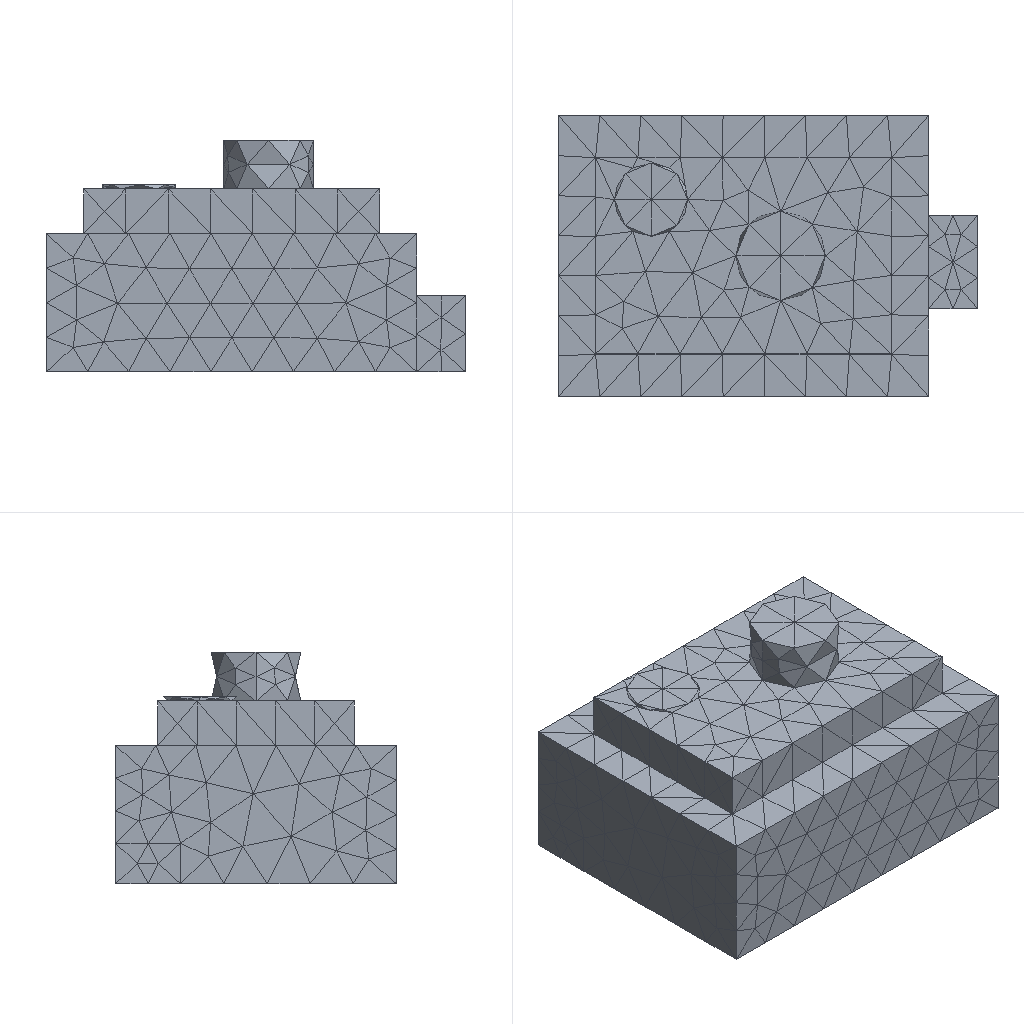Simulation study | ansys mapdl
Set-up summary:
category,name,step,type,value,unit,region
solver,ansys_mapdl
units,mm-N-s-tonne (MPa),,inferred,E=210000 density=
analysis,model,,static
mesh,nodes,,,4047
mesh,elements,,,2393
element_type,SOLID187,,,2393
material,mat 1,,E,210000
material,mat 1,,nu,0.3
load,,model,body load temp,,,all
load,,model,force,"1000 [dir=(0, 0, -1) n=141]",,node list
bc,,model,fixed,"[dofs=UX,UY,UZ n=4568]",,node list
Ansys APDL input file, long lists of numbers shortened:
/COM,ANSYS RELEASE 2026 R1           BUILD 26.1      UP20260202       09:10:33
/PREP7
/NOPR
/TITLE,2
ANTYPE, 0
*IF,_CDRDOFF,EQ,1,THEN     !if solid model was read in
_CDRDOFF=             !reset flag, numoffs already performed
*ELSE              !offset database for the following FE model
NUMOFF,NODE,     4047
NUMOFF,ELEM,     2393
NUMOFF,MAT ,        1
NUMOFF,TYPE,        1
*ENDIF
*SET,_RETURN ,  0.
*SET,_STATUS ,  0.
*SET,_UIQR   ,  141.
*SET,__FLOATPARAMETER__,  4047.
DOF,DELETE
ETBLOCK,        1,        1
(2i9,19a9)
        1      187        0        0        0        0        0        0        0        0        0        0        0        0        0        0        0        0        0        0        0
       -1
NBLOCK,6,SOLID,      4047,      4047
(3i9,6e21.13e3)
        1        0        0-2.9525000000000E+001 3.4500000000000E+001 1.0000000000000E+001
! (4046 more lines like these left out)
N,UNBL,LOC,       -1,
EBLOCK,19,SOLID,      2393,      2393
(19i10)
         1         1         1         1         0         0         0         0        10         0         1      1615      1616      1617      1618      1836      1837      1838      1839
! (4785 more lines like these left out)
        -1
MPTEMP,UNBL, 1, 1,  0.    ,
MPDATA,UNBL, 1,EX  ,       1, 1,  210000.000    ,
MPTEMP,UNBL, 1, 1,  0.    ,
MPDATA,UNBL, 1,NUXY,       1, 1, 0.3    ,
MPTEMP,UNBL, 1, 1,  0.    ,
MPDATA,UNBL, 1,PRXY,       1, 1, 0.3    ,
EXTOPT,ATTR,      0,      0,      0
EXTOPT,ESIZE,  0,  0.
EXTOPT,ACLEAR,      0
TREF,  0.
IRLF,  0
BFUNIF,TEMP,_TINY
ACEL,  0.    ,  0.    ,  0.
OMEGA,  0.    ,  0.    ,  0.
DOMEGA,  0.    ,  0.    ,  0.
CGLOC,  0.    ,  0.    ,  0.
CGOMEGA,  0.    ,  0.    ,  0.
DCGOMG,  0.    ,  0.    ,  0.
KUSE,     0
TIME,  0.
ALPHAD,  0.
BETAD,  0.
DMPRAT,  0.
DMPSTR,  0.
CRPLIM, 0.1    ,   0
CRPLIM,  0.    ,   1
NCNV,     0, 1.000000000E+12,     0,  0.    ,  0.
NEQIT,     0
ERESX,DEFA
DBLOCK,      4568
(i9,a6,2(pg16.9))
        1  UX    0.00000000      0.00000000
! (4567 more lines like these left out)
       -1
FBLOCK,       141
(i9,a6,2(pg16.9))
      802  FZ   -7.09219858      0.00000000
! (140 more lines like these left out)
       -1
/GO
FINISH
Results summary:
result,analysis_type_db,,,static,unstated
result,n_sets,,,1,unstated
result,load_steps[0].set,load_step=1,,1,unstated
result,load_steps[0].substep,load_step=1,,1,unstated
result,load_steps[0].time,load_step=1,,1,unstated
result,load_steps[0].freq,load_step=1,,1,unstated
result,load_steps[0].max_usum,load_step=1,,0.0003283,unstated
result,load_steps[0].max_seqv,load_step=1,,3.803,unstated
result,load_steps[0].reaction_sum.FX,load_step=1,,-4.56894e-12,unstated
result,load_steps[0].reaction_sum.FY,load_step=1,,-1.38272e-11,unstated
result,load_steps[0].reaction_sum.FZ,load_step=1,,1000,unstated
result,load_steps[0].reaction_sum.MX,load_step=1,,0,unstated
result,load_steps[0].reaction_sum.MY,load_step=1,,0,unstated
result,load_steps[0].reaction_sum.MZ,load_step=1,,0,unstated
result,convergence,,,results present for all listed sets,unstated